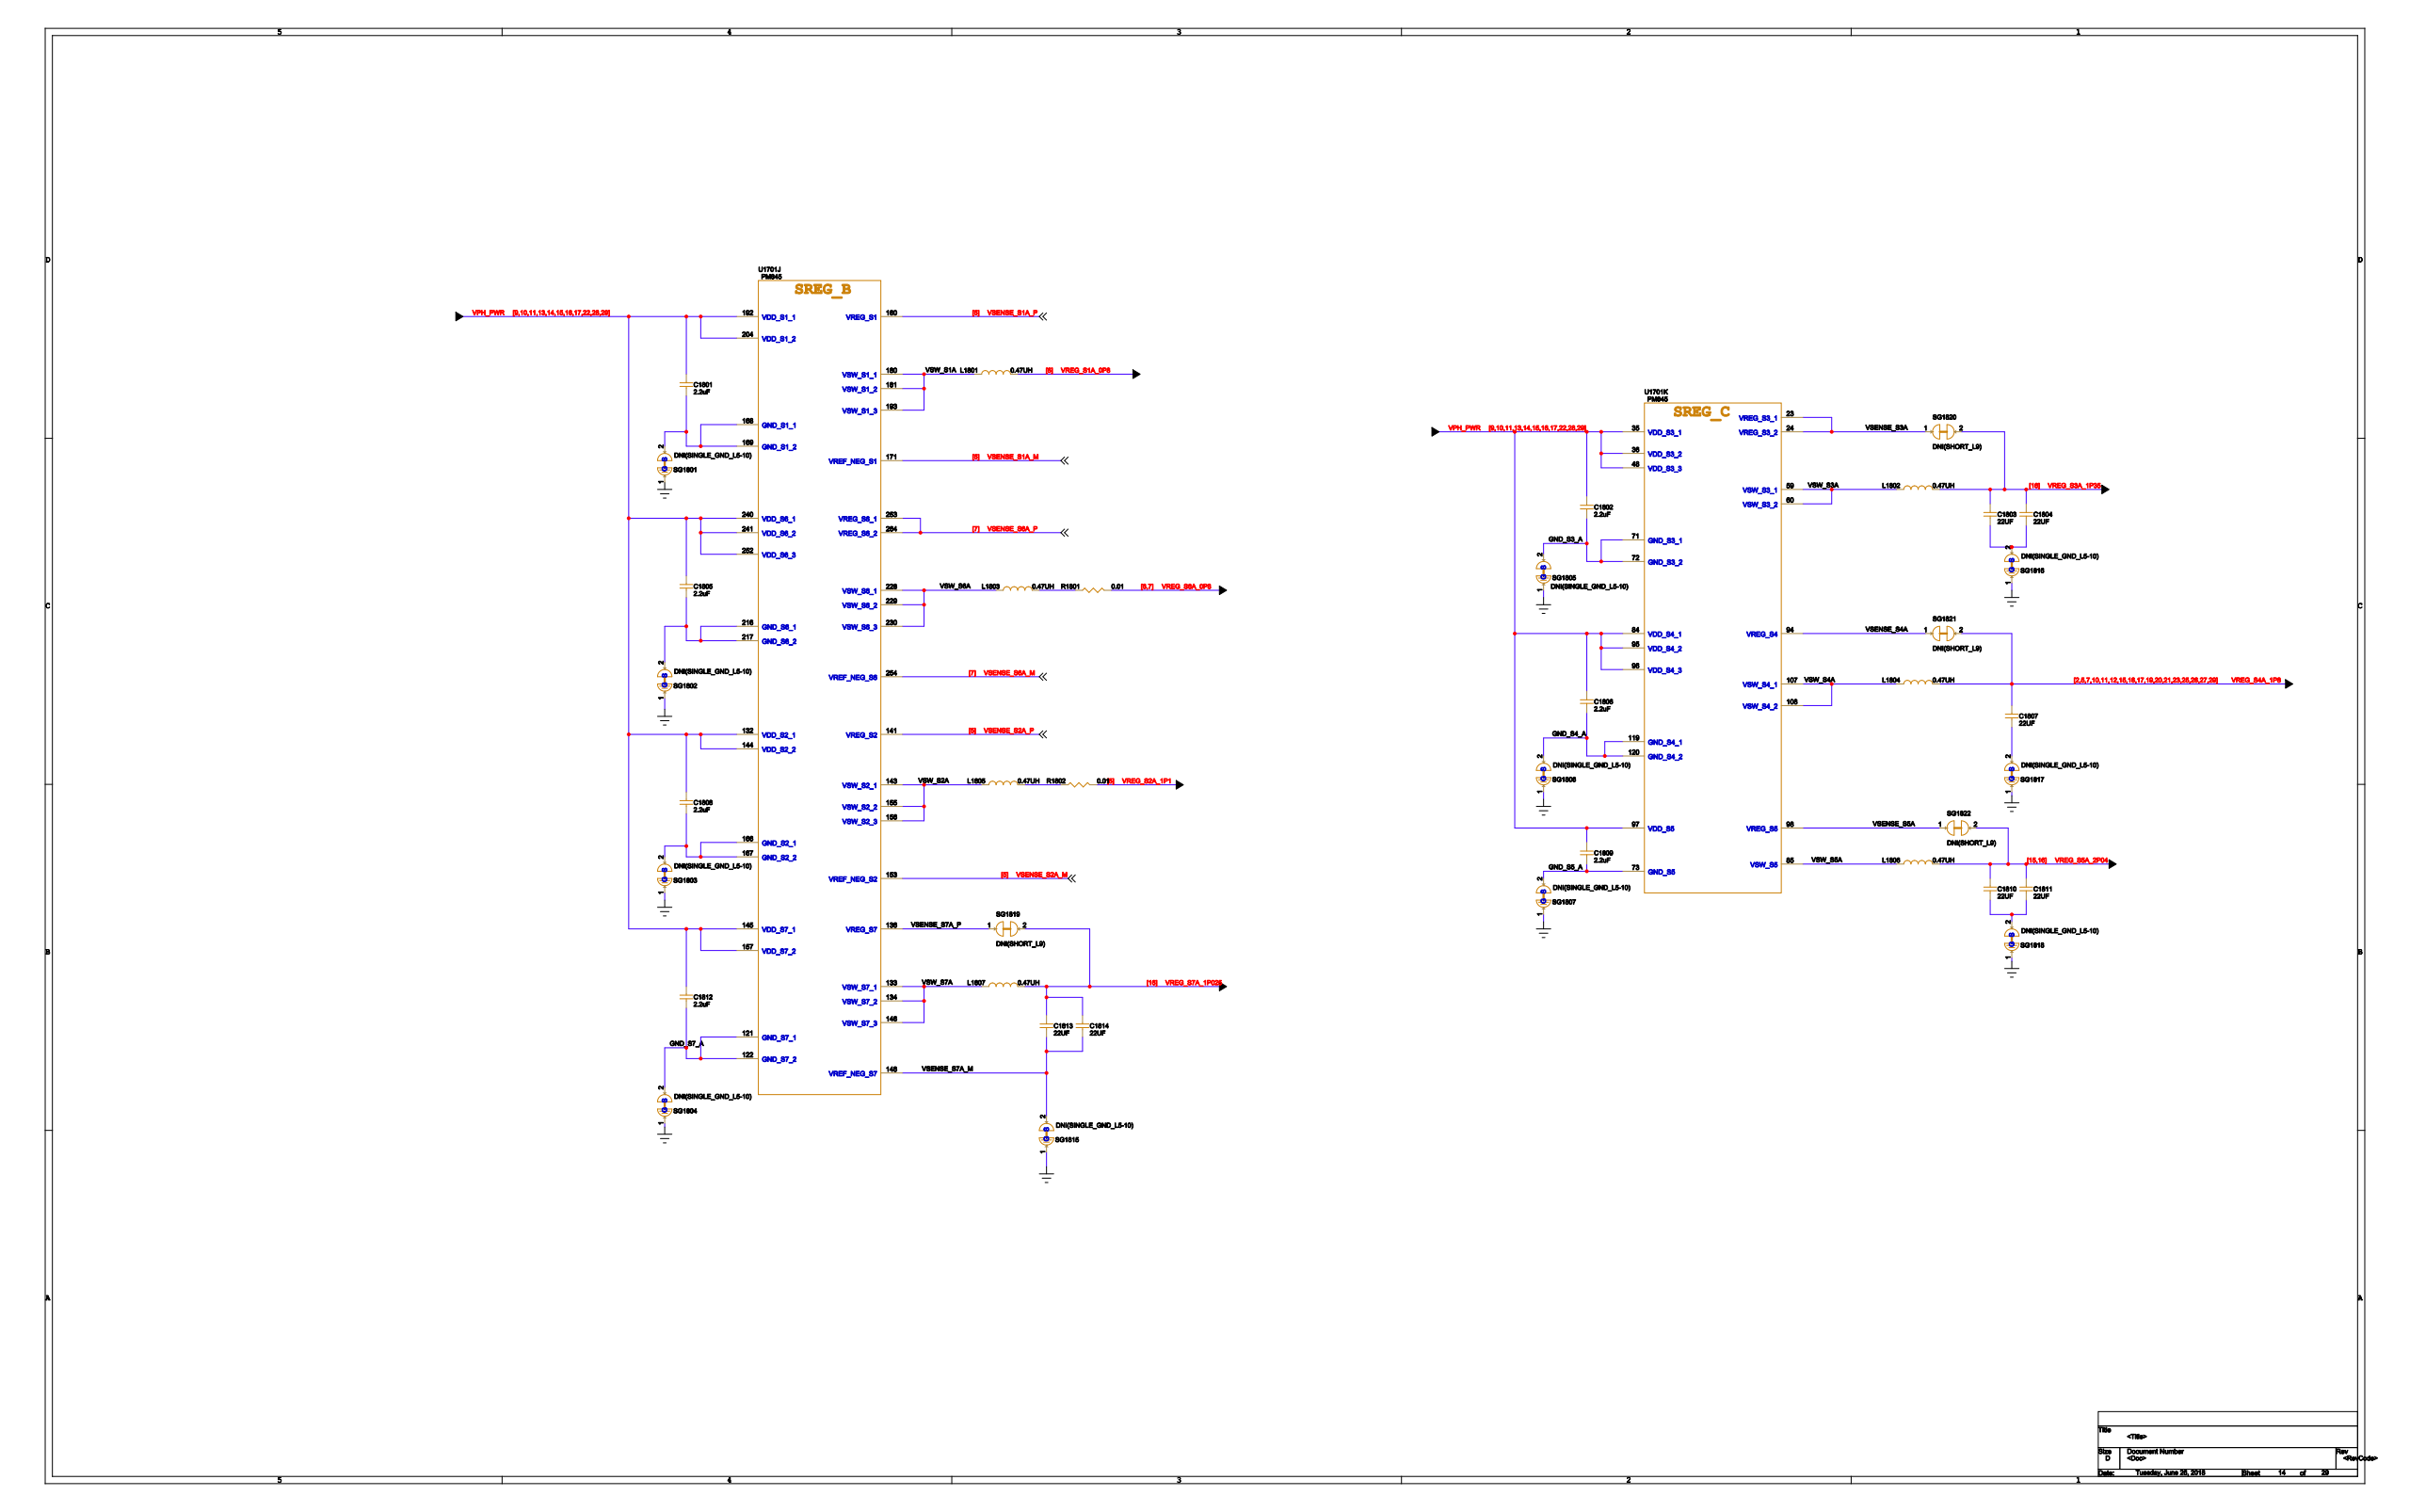Circuit board | Cadence Allegro | 802 parts | 566 nets | one sheet of the schematic
Parts on this sheet (reference | value | footprint):
C1801 | 2.2uF | 0402-BIG
C1802 | 2.2uF | 0402-BIG
C1803 | 22UF | 0603-BIG
C1804 | 22UF | 0603-BIG
C1805 | 2.2uF | 0402-BIG
C1806 | 2.2uF | 0402-BIG
C1807 | 22UF | 0603-BIG
C1808 | 2.2uF | 0402-BIG
C1809 | 2.2uF | 0402-BIG
C1810 | 22UF | 0603-BIG
C1811 | 22UF | 0603-BIG
C1812 | 2.2uF | 0402-BIG
C1813 | 22UF | 0603-BIG
C1814 | 22UF | 0603-BIG
L1801 | 0.47UH | L2016_MEKK2016
L1802 | 0.47UH | L2016_MEKK2016
L1803 | 0.47UH | L2016_MEKK2016
L1804 | 0.47UH | L2016_MEKK2016
L1805 | 0.47UH | L2016_MEKK2016
L1806 | 0.47UH | L2016_MEKK2016
L1807 | 0.47UH | L2016_MEKK2016
R1801 | 0.01 | R0603
R1802 | 0.01 | R0603
SG1801 | DNI(SINGLE_GND_L5-10) | GND_L5-10
SG1802 | DNI(SINGLE_GND_L5-10) | GND_L5-10
SG1803 | DNI(SINGLE_GND_L5-10) | GND_L5-10
SG1804 | DNI(SINGLE_GND_L5-10) | GND_L5-10
SG1805 | DNI(SINGLE_GND_L5-10) | GND_L5-10
SG1806 | DNI(SINGLE_GND_L5-10) | GND_L5-10
SG1807 | DNI(SINGLE_GND_L5-10) | GND_L5-10
SG1815 | DNI(SINGLE_GND_L5-10) | GND_L5-10
SG1816 | DNI(SINGLE_GND_L5-10) | GND_L5-10
SG1817 | DNI(SINGLE_GND_L5-10) | GND_L5-10
SG1818 | DNI(SINGLE_GND_L5-10) | GND_L5-10
SG1819 | DNI(SHORT_L9) | SHORT_L9_2REC08X12
SG1820 | DNI(SHORT_L9) | SHORT_L9_2REC08X12
SG1821 | DNI(SHORT_L9) | SHORT_L9_2REC08X12
SG1822 | DNI(SHORT_L9) | SHORT_L9_2REC08X12
U1701 | PM845 | PM8998
Nets of these parts (net: part-pin ...):
GND: SG1801-1 SG1802-1 SG1803-1 SG1804-1 SG1805-1 SG1806-1 SG1807-1 SG1815-1 SG1816-1 SG1817-1 SG1818-1 U1701-7
VPH_PWR: C1801-1 C1802-1 C1805-1 C1806-1 C1808-1 C1809-1 C1812-1 U1701-35 U1701-36 U1701-48 U1701-84 U1701-95 U1701-96 U1701-97 U1701-132 U1701-144 U1701-145 U1701-157 U1701-192 U1701-204 U1701-240 U1701-241 U1701-252
VREG_S4A_1P8: C1807-1 L1804-2 SG1821-2
VREG_S6A_0P8: R1801-2
VREG_S2A_1P1: R1802-2
N214233: L1803-2 R1801-1
N206765: L1805-2 R1802-1
VREG_S1A_0P8: L1801-2
VREG_S3A_1P35: C1803-1 C1804-1 L1802-2 SG1820-2 U1701-22
N207521: C1803-2 C1804-2 SG1816-2
N207533: C1807-2 SG1817-2
VREG_S5A_2P04: C1810-1 C1811-1 L1806-2 SG1822-2 U1701-29
N207537: C1810-2 C1811-2 SG1818-2
VREG_S7A_1P025: C1813-1 C1814-1 L1807-2 SG1819-2
VSENSE_S7A_M: C1813-2 C1814-2 SG1815-2 U1701-148
N210223: C1801-2 SG1801-2 U1701-168 U1701-169
GND_S3_A: C1802-2 SG1805-2 U1701-71 U1701-72
N209920: C1805-2 SG1802-2 U1701-216 U1701-217
GND_S4_A: C1806-2 SG1806-2 U1701-119 U1701-120
N209551: C1808-2 SG1803-2 U1701-166 U1701-167
GND_S5_A: C1809-2 SG1807-2 U1701-73
GND_S7_A: C1812-2 SG1804-2 U1701-121 U1701-122
VSW_S1A: L1801-1 U1701-180 U1701-181 U1701-193
VSW_S3A: L1802-1 U1701-59 U1701-60
VSW_S6A: L1803-1 U1701-228 U1701-229 U1701-230
VSW_S4A: L1804-1 U1701-107 U1701-108
VSW_S2A: L1805-1 U1701-143 U1701-155 U1701-156
VSW_S5A: L1806-1 U1701-85
VSW_S7A: L1807-1 U1701-133 U1701-134 U1701-146
VSENSE_S2A_M: U1701-153
VSENSE_S2A_P: U1701-141
VSENSE_S1A_M: U1701-171
VSENSE_S1A_P: U1701-160
VSENSE_S6A_M: U1701-254
VSENSE_S6A_P: U1701-253 U1701-264
VSENSE_S7A_P: SG1819-1 U1701-136
VSENSE_S3A: SG1820-1 U1701-23 U1701-24
VSENSE_S4A: SG1821-1 U1701-94
VSENSE_S5A: SG1822-1 U1701-98